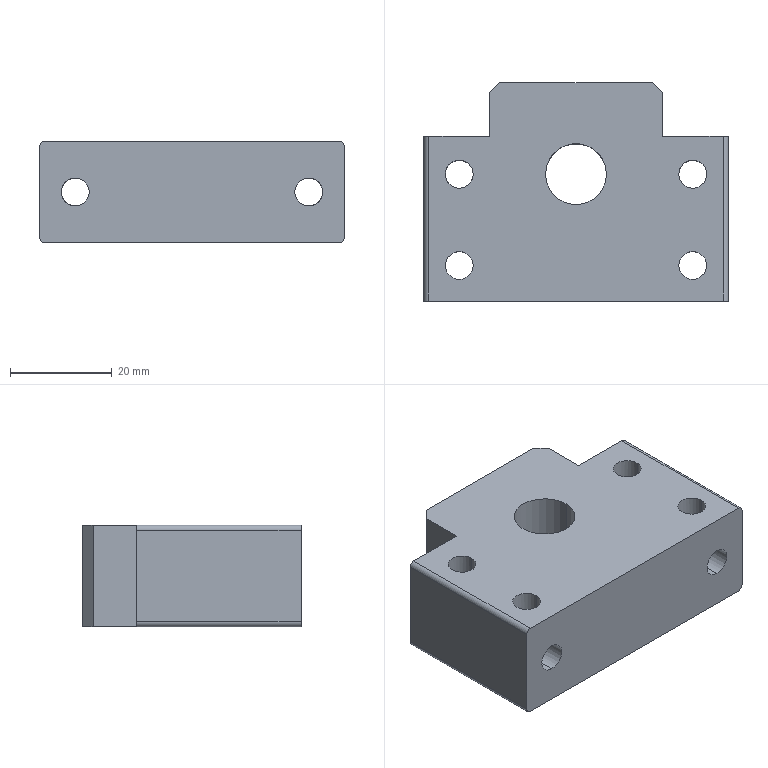Part | SolidWorks | features BaseBody 1 | 1 solid | 56 faces | box 60 x 43 x 20 mm | volume 40698 mm3 | cylinder 38 | plane 14 | cone 4 | commonest cylinder face diameters 5.5 x28 2 x4 11 x4 12 x2